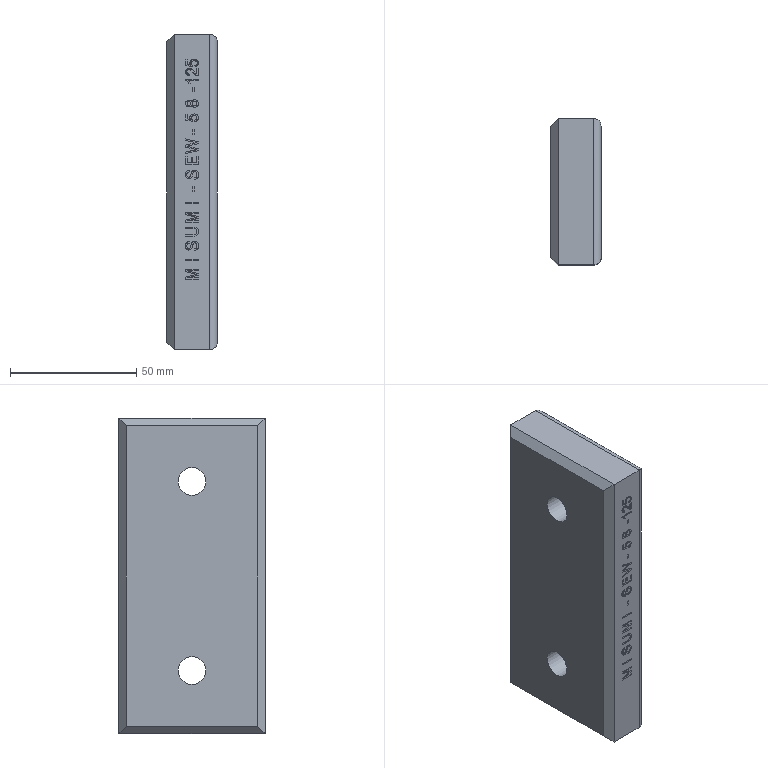Part | STEP file | lll_id4242_x_t | 1 solid | 301 faces | box 20 x 58 x 125 mm | volume 135294 mm3 | other 174 | plane 117 | cylinder 8 | torus 2 | commonest cylinder face diameters 6 x4 11 x2 17.5 x2